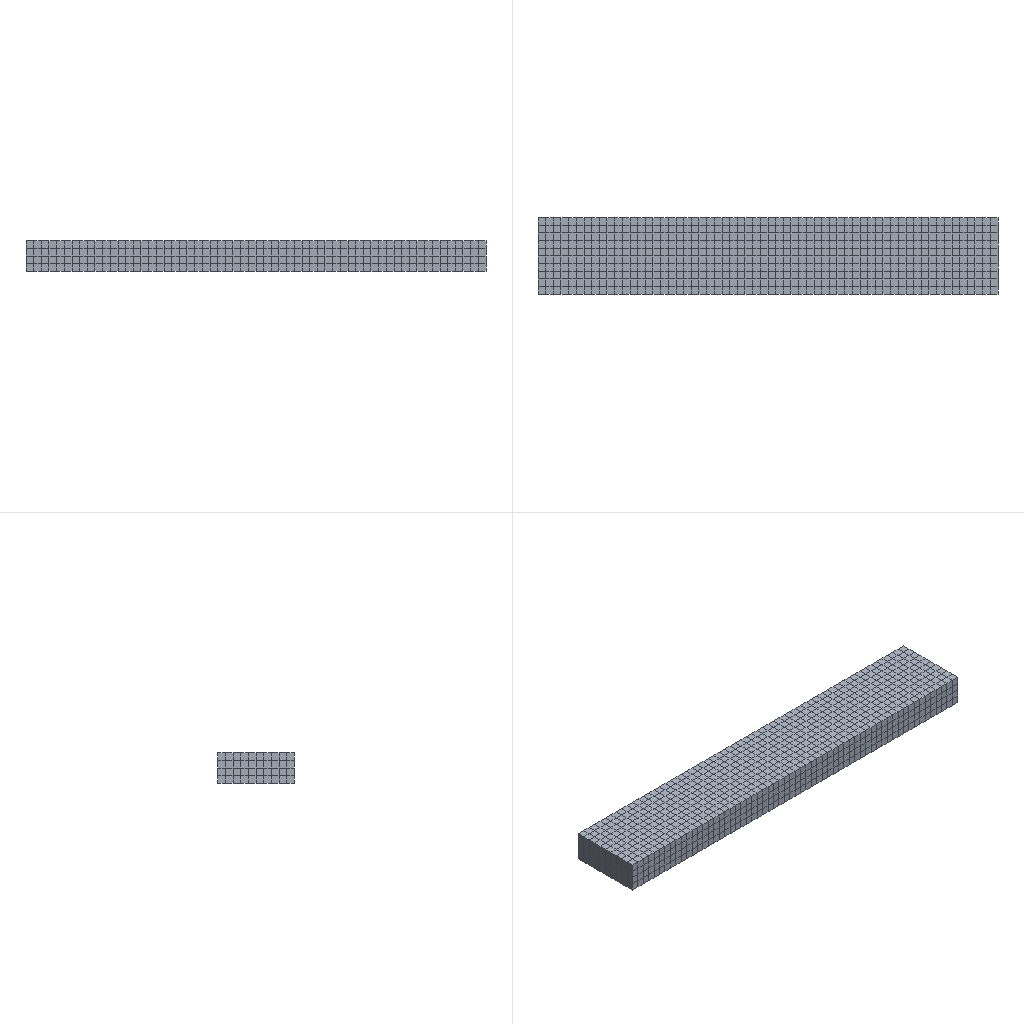Simulation study | ansys workbench
Set-up summary:
category,name,step,type,value,unit,region
solver,ansys_mapdl
solver,version,,,22.2
units,MPA,,stated
analysis,deck,,static,static
load_step,requested,,,1
analysis,nlgeom,,,False
mesh,nodes,,,12389
mesh,elements,,,3000
element_type,ANSYS 186 (type 1),,solid,2400
element_type,ANSYS 154 (type 2),,surface,600
load,load commands in deck,,count,3
bc,support commands in deck,,count,1
named_set,_FIXEDSU,,component
material,1,,in results
check,setup vs results,,match,600 surface effect element(s) are not in the reader's mesh and were not compared
Ansys APDL input file, long lists of numbers shortened:
/batch
/config,noeldb,1     ! force off writing results to database
*get,_wallstrt,active,,time,wall
! ANSYS input file written by Workbench version 2022 R2
! File used for geometry attach: D:\虚拟C盘\长方体.STEP
/title,___--____ (A5)
! ****** Begin Custom Load Command Snippet ******
/COM, ACT Extensions:
/COM,     LSDYNA, 2022.2
/COM,/COM,     ANSYSMotion, 2022.2
/COM,
! ****** End   Custom Load Command Snippet ******
*DIM,_wb_ProjectScratch_dir,string,248
_wb_ProjectScratch_dir(1) = 'D:\虚拟C盘\长方体\_ProjectScratch\ScrC196\'
*DIM,_wb_SolverFiles_dir,string,248
_wb_SolverFiles_dir(1) = 'D:\虚拟C盘\长方体\长方体_files\dp0\SYS\MECH\'
*DIM,_wb_userfiles_dir,string,248
_wb_userfiles_dir(1) = 'D:\虚拟C盘\长方体\长方体_files\user_files\'
/com,--- Data in consistent NMM units. See Solving Units in the help system for more information.
/units,MPA
/nopr
/wb,file,start              !  signify a WB generated input file
/prep7
! Turn off shape checking because checks already performed inside WB mesher.
! See help system for more information.
SHPP,OFF,,NOWARN
/nolist
etcon,set             ! allow ANSYS to choose best KEYOP's for 180x elements, resets any applicable keyopt to MAPDL defaults
/com,*********** Nodes for the whole assembly ***********
nblock,3,,13627
(1i9,3e20.9e3)
        1     1.312500000E+01     7.994791667E+01     1.000000000E+01
! (12388 more lines like these left out)
-1
/wb,elem,start            !  set before creation of elements
/com,*********** Elements for Body 1 "___-FreeParts|__-__1" ***********
et,1,186
keyo,1,2,1          ! set full integration on SOLID186
eblock,19,solid,,2400
(19i9)
        1        1        1        1        0        0        0        0       20        0        1        6        9      180      177      716      713      731      734
! (4799 more lines like these left out)
-1
/wb,elem,end               !  done creating elements
/com,*********** Send User Defined Coordinate System(s) ***********
csys,0
toffst,273.15,  ! Temperature offset from absolute zero
/com,*********** Set Reference Temperature ***********
tref,22.
/wb,mat,start              !  starting to send materials
/com,*********** Send Materials ***********
Temperature = 'TEMP' ! Temperature
MP,DENS,1,7.85e-09,	! tonne mm^-3
MP,ALPX,1,1.2e-05,	! C^-1
MP,C,1,434000000,	! mm^2 s^-2 C^-1
MP,KXX,1,60.5,	! tonne mm s^-3 C^-1
MP,RSVX,1,0.00017,	! ohm mm
MP,EX,1,206000,	! tonne s^-2 mm^-1
MP,NUXY,1,0.3,
MP,MURX,1,10000,
/wb,mat,end                !  done sending materials
!************************* Model Summary ********************
!___-FreeParts|__-__1,	Q235钢,	matid,	1
!************************* End Model Summary ********************
! get the diagonal of the bounding box. Needed later for other things
*get,_xmin,node,,mnloc,x
*get,_ymin,node,,mnloc,y
*get,_zmin,node,,mnloc,z
*get,_xmax,node,,mxloc,x
*get,_ymax,node,,mxloc,y
*get,_zmax,node,,mxloc,z
_ASMDIAG=(_xmax-_xmin)*(_xmax-_xmin)+(_ymax-_ymin)*(_ymax-_ymin)+(_zmax-_zmin)*(_zmax-_zmin)
_ASMDIAG=SQRT(_ASMDIAG)
/wb,contact,start          !  starting to send contact
/wb,contact,end            !  done creating contacts
/golist
/wb,load,start             !  starting to send loads
/com,*********** Fixed Supports ***********
CMBLOCK,_FIXEDSU,NODE,      149
(8i10)
      2131      2162      2205      2206      2207      2218      2219      2223
! (18 more lines like these left out)
cmsel,s,_FIXEDSU
d,all,all
nsel,all
/com,*********** Define Pressure Vector Using Surface Effect Elements ***********
local,12,0,0.,0.,0.,0.,0.,0.
csys,0
et,2,154
eblock,10,,,600
(15i9)
     4161        2        2        2       12     2089     1677     1595     1594     9104     8875     8870     8873
! (599 more lines like these left out)
-1
esel,s,type,,2
keyop,2,2,1                ! Apply load in local coordinate system
keyop,2,7,0                ! Use deformed area for application of load
esel,all
/gst,on,on
fini
*get,_numnode,node,0,count
*get,_numelem,elem,0,count
*get, _MAXELEMNUM, elem, 0, NUM, MAX
*get, _MAXNODENUM, node, 0, NUM, MAX
*get, _MAXELEMTYPE, etyp, 0, NUM, MAX
*get, _MAXREALCONST, rcon, 0, NUM, MAX
/go
/wb,load,end               !  done creating loads
/com,--- Number of total nodes = %_numnode%
/com,--- Number of contact elements = 600
/com,--- Number of spring elements = 0
/com,--- Number of bearing elements = 0
/com,--- Number of solid elements = 2400
/com,--- Number of condensed parts = 0
/com,--- Number of total elements = %_numelem%
*get,_wallbsol,active,,time,wall
/com,****************************************************************************
/com,*************************    SOLUTION       ********************************
/com,****************************************************************************
/solu
antype,0                   ! static analysis
_thickRatio=  1     ! Ratio of thick parts in the model
eqsl,pcg,1e-8,,,,,,1
cntr,print,1               ! print out contact info and also make no initial contact an error
dmpoption,emat,no             ! Don't combine emat file for DANSYS
dmpoption,esav,no             ! Don't combine esav file for DANSYS
nldiag,cont,iter           ! print out contact info each equilibrium iteration
rescontrol,,none                 ! Do not keep any restart files
/com,****************************************************
/com,******************* SOLVE FOR LS 1 OF 1 ****************
esel,s,type,,2
nsle
sfe,all,1,pres,1,0.
sfe,all,2,pres,1,0.
sfe,all,3,pres,1,7.8
nsel,all
esel,all
/nopr
/gopr
nsub,1,1,1
time,1.
outres,erase
outres,all,none
outres,nsol,all,
outres,rsol,all
outres,eangl,all
outres,etmp,all
outres,veng,all
outres,strs,all,
outres,epel,all,
outres,eppl,all,
outres,cont,all,
! *********** WB SOLVE COMMAND ***********
! check interactive state
*get,ANSINTER_,active,,int
*if,ANSINTER_,ne,0,then
/eof
*endif
solve
/com *************** Write FE CONNECTORS *********
CEWRITE,file,ce,,INTE
/com,****************************************************
/com,*************** FINISHED SOLVE FOR LS 1 *************
*get,_wallasol,active,,time,wall
/nopr
*get,_numnode,node,0,count
*get,_numelem,elem,0,count
*get, _MAXELEMNUM, elem, 0, NUM, MAX
*get, _MAXNODENUM, node, 0, NUM, MAX,,,INTERNAL
*get, _MAXELEMTYPE, etyp, 0, NUM, MAX
*get, _MAXREALCONST, rcon, 0, NUM, MAX
*get,_NSOLTHREADS,active,0,ntfs
*get,_NSOLPROCESSES,active,0,npfs
/gopr
*get,_PCGITER,active,,solu,cgiter
/post1
xmlo,ENCODING,ISO-8859-1
xmlo,parm
/xml,parm,xml
fini
/gopr
*get,_walldone,active,,time,wall
_preptime=(_wallbsol-_wallstrt)*3600
_solvtime=(_wallasol-_wallbsol)*3600
_posttime=(_walldone-_wallasol)*3600
_totaltim=(_walldone-_wallstrt)*3600
*get,_dlbratio,active,0,solu,dlbr
*get,_combtime,active,0,solu,comb
*get,_ssmode,active,0,solu,ssmm
*get,_ndofs,active,0,solu,ndof
*get,_sol_end_time,active,0,set,time
*if,_sol_end_time,eq,1.,then
/fclean				!clean distributed files
*endif
/com,--- Total number of nodes = %_numnode%
/com,--- Total number of elements = %_numelem%
/com,--- Element load balance ratio = %_dlbratio%
/com,--- Time to combine distributed files = %_combtime%
/com,--- Sparse memory mode = %_ssmode%
/com,--- Number of DOF = %_ndofs%
/wb,file,end               ! done with WB generated input
Results summary:
result,analysis,,,static
result,last_loadstep,,,1
result,primary field,,,displacement
result,reaction total,1,FX,-0.0112,N
result,reaction total,1,FY,-0.002586,N
result,reaction total,1,FZ,-117000,N
result,mass,,,0.002355,"NMM: mm, ton, N, s, mV, mA, degC"